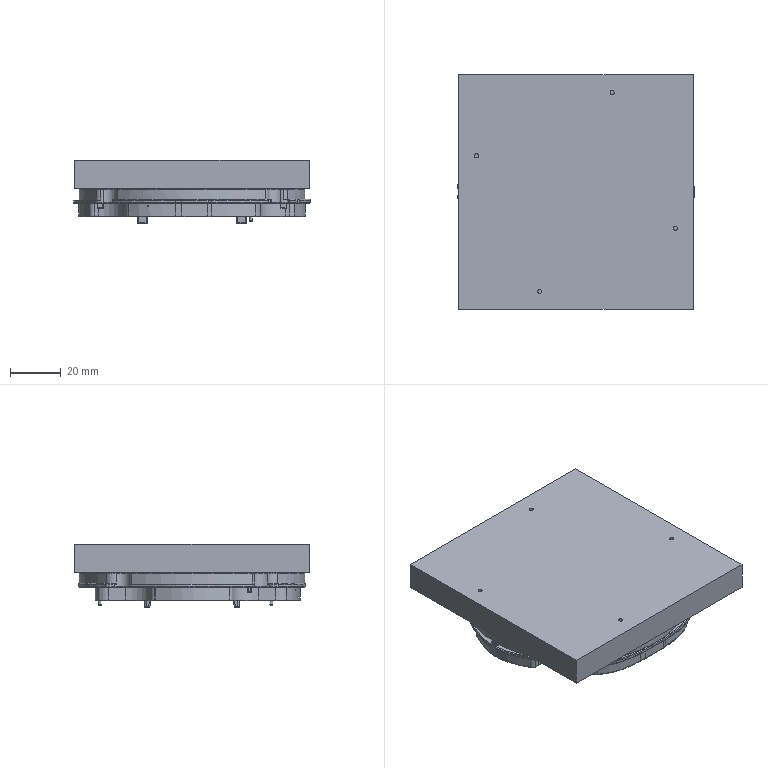NC program | NX | posted with a generic post | part box 92.935 x 92.1 x 24.829 mm
Lines 2410 to 2469 of 7643:
(DRILLING , TOOL : 倒角D4-90度)
N4818 T11 M6
N4820 G53
N4822 G17 G0 G90 X-35.738 Y19.962 S2500 M3
N4824 G43 Z21. H11
N4826 G94 G81 G99 Z-1. F200. R3.
N4828 X14.16 Y39.009
N4830 X35.669 Y19.962
N4832 X38.963 Y-14.182
N4834 X35.669 Y-19.938
N4836 X-14.228 Y-38.985
N4838 X-35.738 Y-19.938
N4840 X-39.031 Y14.206
N4842 G80
N4844 G0 X-39.031 Y14.206 Z21.
N4846 M5
(DRILLING_1 , TOOL : 钻头D2.5-35-61)
N4848 T12 M6
N4850 G53
N4852 G17 G0 G90 X-35.738 Y19.962 S2500 M3
N4854 G43 Z21. H12
N4856 G94 G81 G99 Z-10. F200. R3.
N4858 X35.669
N4860 Y-19.938
N4862 X-35.738
N4864 G80
N4866 G0 X-35.738 Y-19.938 Z21.
N4868 M5
(DRILLING_2 , TOOL : 钻头D1.84-11-D3-40)
N4870 T13 M6
N4872 G53
N4874 G17 G0 G90 X-39.031 Y14.206 S1800 M3
N4876 G43 Z21. H13
N4878 G94 G83 G99 Z-5.6 F120. Q1. R3.
N4880 X14.16 Y39.009
N4882 X38.963 Y-14.182
N4884 X-14.228 Y-38.985
N4886 G80
N4888 G0 X-14.228 Y-38.985 Z21.
N4890 M5
(DRILLING_2_COPY , TOOL : 挤压M2-12-D3-39)
N4892 T14 M6
N4894 G53
N4896 G17 G0 G90 X-39.031 Y14.206 S300 M3
N4898 G43 Z21. H14
N4900 G84 G94 G99 Z-5. F120. R3.
N4902 X14.16 Y39.009
N4904 X38.963 Y-14.182
N4906 X-14.228 Y-38.985
N4908 G80
N4910 G0 X-14.228 Y-38.985 Z21.
N4912 M5